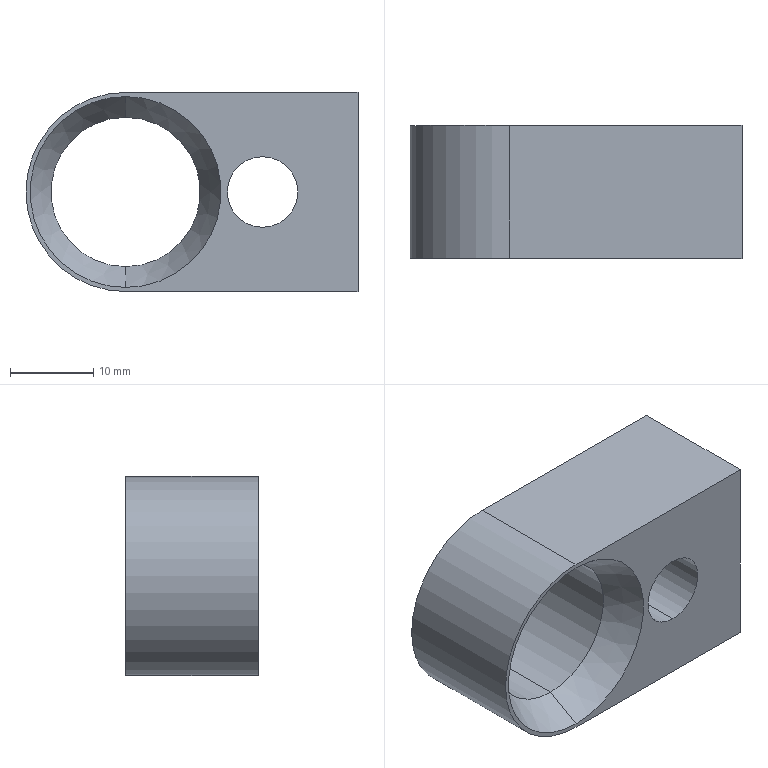Part | 1 solid | 12 faces | box 40 x 16 x 24 mm | volume 9057 mm3 | cylinder 5 | plane 5 | cone 2 | commonest cylinder face diameters 8.5 x2 18 x2 24 x1
STEP:
#1=CARTESIAN_POINT('',(-8.,4.33,9.));
#2=VERTEX_POINT('',#1);
#3=CARTESIAN_POINT('',(-8.,4.33,-9.));
#4=VERTEX_POINT('',#3);
#5=CARTESIAN_POINT('',(-8.,4.33,0.));
#6=DIRECTION('',(0.,1.,0.));
#7=DIRECTION('',(0.,0.,-1.));
#8=AXIS2_PLACEMENT_3D('',#5,#6,#7);
#9=CIRCLE('',#8,9.);
#10=EDGE_CURVE('',#2,#4,#9,.T.);
#11=ORIENTED_EDGE('',*,*,#10,.T.);
#12=CARTESIAN_POINT('',(-8.,0.,-11.5));
#13=VERTEX_POINT('',#12);
#14=CARTESIAN_POINT('',(-8.,0.,-11.5));
#15=DIRECTION('',(0.,-0.866,-0.5));
#16=VECTOR('',#15,1000.);
#17=LINE('',#14,#16);
#18=EDGE_CURVE('',#4,#13,#17,.T.);
#19=ORIENTED_EDGE('',*,*,#18,.T.);
#20=CARTESIAN_POINT('',(-8.,0.,11.5));
#21=VERTEX_POINT('',#20);
#22=CARTESIAN_POINT('',(-8.,0.,0.));
#23=DIRECTION('',(0.,1.,0.));
#24=DIRECTION('',(0.,0.,1.));
#25=AXIS2_PLACEMENT_3D('',#22,#23,#24);
#26=CIRCLE('',#25,11.5);
#27=EDGE_CURVE('',#21,#13,#26,.T.);
#28=ORIENTED_EDGE('',*,*,#27,.F.);
#29=CARTESIAN_POINT('',(-8.,0.,11.5));
#30=DIRECTION('',(0.,-0.866,0.5));
#31=VECTOR('',#30,1000.);
#32=LINE('',#29,#31);
#33=EDGE_CURVE('',#2,#21,#32,.T.);
#34=ORIENTED_EDGE('',*,*,#33,.F.);
#35=EDGE_LOOP('',(#11,#19,#28,#34));
#36=FACE_OUTER_BOUND('',#35,.T.);
#37=CARTESIAN_POINT('',(-8.,0.,0.));
#38=DIRECTION('',(0.,-1.,0.));
#39=DIRECTION('',(0.,0.,1.));
#40=AXIS2_PLACEMENT_3D('',#37,#38,#39);
#41=CONICAL_SURFACE('',#40,11.5,0.5236);
#42=ADVANCED_FACE('',(#36),#41,.F.);
#43=CARTESIAN_POINT('',(8.5,0.,-4.25));
#44=VERTEX_POINT('',#43);
#45=CARTESIAN_POINT('',(8.5,0.,4.25));
#46=VERTEX_POINT('',#45);
#47=CARTESIAN_POINT('',(8.5,0.,0.));
#48=DIRECTION('',(0.,1.,0.));
#49=DIRECTION('',(0.,0.,1.));
#50=AXIS2_PLACEMENT_3D('',#47,#48,#49);
#51=CIRCLE('',#50,4.25);
#52=EDGE_CURVE('',#44,#46,#51,.T.);
#53=ORIENTED_EDGE('',*,*,#52,.F.);
#54=CARTESIAN_POINT('',(8.5,16.,-4.25));
#55=VERTEX_POINT('',#54);
#56=CARTESIAN_POINT('',(8.5,0.,-4.25));
#57=DIRECTION('',(0.,1.,0.));
#58=VECTOR('',#57,1000.);
#59=LINE('',#56,#58);
#60=EDGE_CURVE('',#44,#55,#59,.T.);
#61=ORIENTED_EDGE('',*,*,#60,.T.);
#62=CARTESIAN_POINT('',(8.5,16.,4.25));
#63=VERTEX_POINT('',#62);
#64=CARTESIAN_POINT('',(8.5,16.,0.));
#65=DIRECTION('',(0.,1.,0.));
#66=DIRECTION('',(0.,0.,1.));
#67=AXIS2_PLACEMENT_3D('',#64,#65,#66);
#68=CIRCLE('',#67,4.25);
#69=EDGE_CURVE('',#55,#63,#68,.T.);
#70=ORIENTED_EDGE('',*,*,#69,.T.);
#71=CARTESIAN_POINT('',(8.5,0.,4.25));
#72=DIRECTION('',(0.,1.,0.));
#73=VECTOR('',#72,1000.);
#74=LINE('',#71,#73);
#75=EDGE_CURVE('',#46,#63,#74,.T.);
#76=ORIENTED_EDGE('',*,*,#75,.F.);
#77=EDGE_LOOP('',(#53,#61,#70,#76));
#78=FACE_OUTER_BOUND('',#77,.T.);
#79=CARTESIAN_POINT('',(8.5,0.,0.));
#80=DIRECTION('',(0.,1.,0.));
#81=DIRECTION('',(0.,0.,1.));
#82=AXIS2_PLACEMENT_3D('',#79,#80,#81);
#83=CYLINDRICAL_SURFACE('',#82,4.25);
#84=ADVANCED_FACE('',(#78),#83,.F.);
#85=CARTESIAN_POINT('',(-8.,4.33,0.));
#86=DIRECTION('',(0.,1.,0.));
#87=DIRECTION('',(0.,0.,-1.));
#88=AXIS2_PLACEMENT_3D('',#85,#86,#87);
#89=CIRCLE('',#88,9.);
#90=EDGE_CURVE('',#4,#2,#89,.T.);
#91=ORIENTED_EDGE('',*,*,#90,.F.);
#92=CARTESIAN_POINT('',(-8.,16.,-9.));
#93=VERTEX_POINT('',#92);
#94=CARTESIAN_POINT('',(-8.,0.,-9.));
#95=DIRECTION('',(0.,1.,0.));
#96=VECTOR('',#95,1000.);
#97=LINE('',#94,#96);
#98=EDGE_CURVE('',#4,#93,#97,.T.);
#99=ORIENTED_EDGE('',*,*,#98,.T.);
#100=CARTESIAN_POINT('',(-8.,16.,9.));
#101=VERTEX_POINT('',#100);
#102=CARTESIAN_POINT('',(-8.,16.,0.));
#103=DIRECTION('',(0.,1.,0.));
#104=DIRECTION('',(0.,0.,1.));
#105=AXIS2_PLACEMENT_3D('',#102,#103,#104);
#106=CIRCLE('',#105,9.);
#107=EDGE_CURVE('',#93,#101,#106,.T.);
#108=ORIENTED_EDGE('',*,*,#107,.T.);
#109=CARTESIAN_POINT('',(-8.,0.,9.));
#110=DIRECTION('',(0.,1.,0.));
#111=VECTOR('',#110,1000.);
#112=LINE('',#109,#111);
#113=EDGE_CURVE('',#2,#101,#112,.T.);
#114=ORIENTED_EDGE('',*,*,#113,.F.);
#115=EDGE_LOOP('',(#91,#99,#108,#114));
#116=FACE_OUTER_BOUND('',#115,.T.);
#117=CARTESIAN_POINT('',(-8.,0.,0.));
#118=DIRECTION('',(0.,1.,0.));
#119=DIRECTION('',(0.,0.,1.));
#120=AXIS2_PLACEMENT_3D('',#117,#118,#119);
#121=CYLINDRICAL_SURFACE('',#120,9.);
#122=ADVANCED_FACE('',(#116),#121,.F.);
#123=ORIENTED_EDGE('',*,*,#98,.F.);
#124=ORIENTED_EDGE('',*,*,#10,.F.);
#125=ORIENTED_EDGE('',*,*,#113,.T.);
#126=CARTESIAN_POINT('',(-8.,16.,0.));
#127=DIRECTION('',(0.,1.,0.));
#128=DIRECTION('',(0.,0.,1.));
#129=AXIS2_PLACEMENT_3D('',#126,#127,#128);
#130=CIRCLE('',#129,9.);
#131=EDGE_CURVE('',#101,#93,#130,.T.);
#132=ORIENTED_EDGE('',*,*,#131,.T.);
#133=EDGE_LOOP('',(#123,#124,#125,#132));
#134=FACE_OUTER_BOUND('',#133,.T.);
#135=CARTESIAN_POINT('',(-8.,0.,0.));
#136=DIRECTION('',(0.,1.,0.));
#137=DIRECTION('',(0.,0.,1.));
#138=AXIS2_PLACEMENT_3D('',#135,#136,#137);
#139=CYLINDRICAL_SURFACE('',#138,9.);
#140=ADVANCED_FACE('',(#134),#139,.F.);
#141=CARTESIAN_POINT('',(8.5,16.,0.));
#142=DIRECTION('',(0.,1.,0.));
#143=DIRECTION('',(0.,0.,1.));
#144=AXIS2_PLACEMENT_3D('',#141,#142,#143);
#145=CIRCLE('',#144,4.25);
#146=EDGE_CURVE('',#63,#55,#145,.T.);
#147=ORIENTED_EDGE('',*,*,#146,.F.);
#148=ORIENTED_EDGE('',*,*,#69,.F.);
#149=EDGE_LOOP('',(#147,#148));
#150=FACE_BOUND('',#149,.T.);
#151=ORIENTED_EDGE('',*,*,#131,.F.);
#152=ORIENTED_EDGE('',*,*,#107,.F.);
#153=EDGE_LOOP('',(#151,#152));
#154=FACE_BOUND('',#153,.T.);
#155=CARTESIAN_POINT('',(-8.,16.,-12.));
#156=VERTEX_POINT('',#155);
#157=CARTESIAN_POINT('',(-8.,16.,12.));
#158=VERTEX_POINT('',#157);
#159=CARTESIAN_POINT('',(-8.,16.,0.));
#160=DIRECTION('',(0.,1.,0.));
#161=DIRECTION('',(0.,0.,1.));
#162=AXIS2_PLACEMENT_3D('',#159,#160,#161);
#163=CIRCLE('',#162,12.);
#164=EDGE_CURVE('',#156,#158,#163,.T.);
#165=ORIENTED_EDGE('',*,*,#164,.T.);
#166=CARTESIAN_POINT('',(20.,16.,12.));
#167=VERTEX_POINT('',#166);
#168=CARTESIAN_POINT('',(-20.,16.,12.));
#169=DIRECTION('',(1.,0.,0.));
#170=VECTOR('',#169,1000.);
#171=LINE('',#168,#170);
#172=EDGE_CURVE('',#158,#167,#171,.T.);
#173=ORIENTED_EDGE('',*,*,#172,.T.);
#174=CARTESIAN_POINT('',(20.,16.,-12.));
#175=VERTEX_POINT('',#174);
#176=CARTESIAN_POINT('',(20.,16.,12.));
#177=DIRECTION('',(0.,0.,-1.));
#178=VECTOR('',#177,1000.);
#179=LINE('',#176,#178);
#180=EDGE_CURVE('',#167,#175,#179,.T.);
#181=ORIENTED_EDGE('',*,*,#180,.T.);
#182=CARTESIAN_POINT('',(-20.,16.,-12.));
#183=DIRECTION('',(-1.,0.,0.));
#184=VECTOR('',#183,1000.);
#185=LINE('',#182,#184);
#186=EDGE_CURVE('',#175,#156,#185,.T.);
#187=ORIENTED_EDGE('',*,*,#186,.T.);
#188=EDGE_LOOP('',(#165,#173,#181,#187));
#189=FACE_OUTER_BOUND('',#188,.T.);
#190=CARTESIAN_POINT('',(0.,16.,0.));
#191=DIRECTION('',(0.,-1.,0.));
#192=DIRECTION('',(0.,0.,-1.));
#193=AXIS2_PLACEMENT_3D('',#190,#191,#192);
#194=PLANE('',#193);
#195=ADVANCED_FACE('',(#150,#154,#189),#194,.F.);
#196=ORIENTED_EDGE('',*,*,#27,.T.);
#197=CARTESIAN_POINT('',(-8.,0.,0.));
#198=DIRECTION('',(0.,1.,0.));
#199=DIRECTION('',(0.,0.,1.));
#200=AXIS2_PLACEMENT_3D('',#197,#198,#199);
#201=CIRCLE('',#200,11.5);
#202=EDGE_CURVE('',#13,#21,#201,.T.);
#203=ORIENTED_EDGE('',*,*,#202,.T.);
#204=EDGE_LOOP('',(#196,#203));
#205=FACE_BOUND('',#204,.T.);
#206=CARTESIAN_POINT('',(8.5,0.,0.));
#207=DIRECTION('',(0.,1.,0.));
#208=DIRECTION('',(0.,0.,1.));
#209=AXIS2_PLACEMENT_3D('',#206,#207,#208);
#210=CIRCLE('',#209,4.25);
#211=EDGE_CURVE('',#46,#44,#210,.T.);
#212=ORIENTED_EDGE('',*,*,#211,.T.);
#213=ORIENTED_EDGE('',*,*,#52,.T.);
#214=EDGE_LOOP('',(#212,#213));
#215=FACE_BOUND('',#214,.T.);
#216=CARTESIAN_POINT('',(-8.,0.,12.));
#217=VERTEX_POINT('',#216);
#218=CARTESIAN_POINT('',(20.,0.,12.));
#219=VERTEX_POINT('',#218);
#220=CARTESIAN_POINT('',(-20.,0.,12.));
#221=DIRECTION('',(1.,0.,0.));
#222=VECTOR('',#221,1000.);
#223=LINE('',#220,#222);
#224=EDGE_CURVE('',#217,#219,#223,.T.);
#225=ORIENTED_EDGE('',*,*,#224,.F.);
#226=CARTESIAN_POINT('',(-8.,0.,-12.));
#227=VERTEX_POINT('',#226);
#228=CARTESIAN_POINT('',(-8.,0.,0.));
#229=DIRECTION('',(0.,1.,0.));
#230=DIRECTION('',(0.,0.,1.));
#231=AXIS2_PLACEMENT_3D('',#228,#229,#230);
#232=CIRCLE('',#231,12.);
#233=EDGE_CURVE('',#227,#217,#232,.T.);
#234=ORIENTED_EDGE('',*,*,#233,.F.);
#235=CARTESIAN_POINT('',(20.,0.,-12.));
#236=VERTEX_POINT('',#235);
#237=CARTESIAN_POINT('',(-20.,0.,-12.));
#238=DIRECTION('',(-1.,0.,0.));
#239=VECTOR('',#238,1000.);
#240=LINE('',#237,#239);
#241=EDGE_CURVE('',#236,#227,#240,.T.);
#242=ORIENTED_EDGE('',*,*,#241,.F.);
#243=CARTESIAN_POINT('',(20.,0.,12.));
#244=DIRECTION('',(0.,0.,-1.));
#245=VECTOR('',#244,1000.);
#246=LINE('',#243,#245);
#247=EDGE_CURVE('',#219,#236,#246,.T.);
#248=ORIENTED_EDGE('',*,*,#247,.F.);
#249=EDGE_LOOP('',(#225,#234,#242,#248));
#250=FACE_OUTER_BOUND('',#249,.T.);
#251=CARTESIAN_POINT('',(0.,0.,0.));
#252=DIRECTION('',(0.,-1.,0.));
#253=DIRECTION('',(0.,0.,-1.));
#254=AXIS2_PLACEMENT_3D('',#251,#252,#253);
#255=PLANE('',#254);
#256=ADVANCED_FACE('',(#205,#215,#250),#255,.T.);
#257=CARTESIAN_POINT('',(-8.,0.,12.));
#258=DIRECTION('',(0.,1.,0.));
#259=VECTOR('',#258,1000.);
#260=LINE('',#257,#259);
#261=EDGE_CURVE('',#217,#158,#260,.T.);
#262=ORIENTED_EDGE('',*,*,#261,.F.);
#263=ORIENTED_EDGE('',*,*,#224,.T.);
#264=CARTESIAN_POINT('',(20.,16.,12.));
#265=DIRECTION('',(0.,-1.,0.));
#266=VECTOR('',#265,1000.);
#267=LINE('',#264,#266);
#268=EDGE_CURVE('',#167,#219,#267,.T.);
#269=ORIENTED_EDGE('',*,*,#268,.F.);
#270=ORIENTED_EDGE('',*,*,#172,.F.);
#271=EDGE_LOOP('',(#262,#263,#269,#270));
#272=FACE_OUTER_BOUND('',#271,.T.);
#273=CARTESIAN_POINT('',(-20.,16.,12.));
#274=DIRECTION('',(0.,0.,-1.));
#275=DIRECTION('',(-1.,0.,0.));
#276=AXIS2_PLACEMENT_3D('',#273,#274,#275);
#277=PLANE('',#276);
#278=ADVANCED_FACE('',(#272),#277,.F.);
#279=ORIENTED_EDGE('',*,*,#247,.T.);
#280=CARTESIAN_POINT('',(20.,16.,-12.));
#281=DIRECTION('',(0.,-1.,0.));
#282=VECTOR('',#281,1000.);
#283=LINE('',#280,#282);
#284=EDGE_CURVE('',#175,#236,#283,.T.);
#285=ORIENTED_EDGE('',*,*,#284,.F.);
#286=ORIENTED_EDGE('',*,*,#180,.F.);
#287=ORIENTED_EDGE('',*,*,#268,.T.);
#288=EDGE_LOOP('',(#279,#285,#286,#287));
#289=FACE_OUTER_BOUND('',#288,.T.);
#290=CARTESIAN_POINT('',(20.,16.,12.));
#291=DIRECTION('',(-1.,0.,0.));
#292=DIRECTION('',(0.,0.,1.));
#293=AXIS2_PLACEMENT_3D('',#290,#291,#292);
#294=PLANE('',#293);
#295=ADVANCED_FACE('',(#289),#294,.F.);
#296=ORIENTED_EDGE('',*,*,#241,.T.);
#297=CARTESIAN_POINT('',(-8.,0.,-12.));
#298=DIRECTION('',(0.,1.,0.));
#299=VECTOR('',#298,1000.);
#300=LINE('',#297,#299);
#301=EDGE_CURVE('',#227,#156,#300,.T.);
#302=ORIENTED_EDGE('',*,*,#301,.T.);
#303=ORIENTED_EDGE('',*,*,#186,.F.);
#304=ORIENTED_EDGE('',*,*,#284,.T.);
#305=EDGE_LOOP('',(#296,#302,#303,#304));
#306=FACE_OUTER_BOUND('',#305,.T.);
#307=CARTESIAN_POINT('',(-20.,16.,-12.));
#308=DIRECTION('',(0.,0.,1.));
#309=DIRECTION('',(1.,0.,0.));
#310=AXIS2_PLACEMENT_3D('',#307,#308,#309);
#311=PLANE('',#310);
#312=ADVANCED_FACE('',(#306),#311,.F.);
#313=ORIENTED_EDGE('',*,*,#164,.F.);
#314=ORIENTED_EDGE('',*,*,#301,.F.);
#315=ORIENTED_EDGE('',*,*,#233,.T.);
#316=ORIENTED_EDGE('',*,*,#261,.T.);
#317=EDGE_LOOP('',(#313,#314,#315,#316));
#318=FACE_OUTER_BOUND('',#317,.T.);
#319=CARTESIAN_POINT('',(-8.,0.,0.));
#320=DIRECTION('',(0.,1.,0.));
#321=DIRECTION('',(0.,0.,1.));
#322=AXIS2_PLACEMENT_3D('',#319,#320,#321);
#323=CYLINDRICAL_SURFACE('',#322,12.);
#324=ADVANCED_FACE('',(#318),#323,.T.);
#325=ORIENTED_EDGE('',*,*,#60,.F.);
#326=ORIENTED_EDGE('',*,*,#211,.F.);
#327=ORIENTED_EDGE('',*,*,#75,.T.);
#328=ORIENTED_EDGE('',*,*,#146,.T.);
#329=EDGE_LOOP('',(#325,#326,#327,#328));
#330=FACE_OUTER_BOUND('',#329,.T.);
#331=CARTESIAN_POINT('',(8.5,0.,0.));
#332=DIRECTION('',(0.,1.,0.));
#333=DIRECTION('',(0.,0.,1.));
#334=AXIS2_PLACEMENT_3D('',#331,#332,#333);
#335=CYLINDRICAL_SURFACE('',#334,4.25);
#336=ADVANCED_FACE('',(#330),#335,.F.);
#337=ORIENTED_EDGE('',*,*,#18,.F.);
#338=ORIENTED_EDGE('',*,*,#90,.T.);
#339=ORIENTED_EDGE('',*,*,#33,.T.);
#340=ORIENTED_EDGE('',*,*,#202,.F.);
#341=EDGE_LOOP('',(#337,#338,#339,#340));
#342=FACE_OUTER_BOUND('',#341,.T.);
#343=CARTESIAN_POINT('',(-8.,0.,0.));
#344=DIRECTION('',(0.,-1.,0.));
#345=DIRECTION('',(0.,0.,1.));
#346=AXIS2_PLACEMENT_3D('',#343,#344,#345);
#347=CONICAL_SURFACE('',#346,11.5,0.5236);
#348=ADVANCED_FACE('',(#342),#347,.F.);
#349=CLOSED_SHELL('',(#42,#84,#122,#140,#195,#256,#278,#295,#312,#324,#336,#348));
#350=MANIFOLD_SOLID_BREP('',#349);
#351=CARTESIAN_POINT('',(0.,0.,0.));
#352=DIRECTION('',(0.,0.,1.));
#353=DIRECTION('',(1.,0.,0.));
#354=AXIS2_PLACEMENT_3D('',#351,#352,#353);
#355=(LENGTH_UNIT()NAMED_UNIT(*)SI_UNIT(.MILLI.,.METRE.));
#356=UNCERTAINTY_MEASURE_WITH_UNIT(LENGTH_MEASURE(0.00001),#355,'','');
#357=(NAMED_UNIT(*)PLANE_ANGLE_UNIT()SI_UNIT($,.RADIAN.));
#358=(NAMED_UNIT(*)SI_UNIT($,.STERADIAN.)SOLID_ANGLE_UNIT());
#359=(GEOMETRIC_REPRESENTATION_CONTEXT(3)GLOBAL_UNCERTAINTY_ASSIGNED_CONTEXT((#356))GLOBAL_UNIT_ASSIGNED_CONTEXT((#355,#357,#358))REPRESENTATION_CONTEXT('',''));
#360=ADVANCED_BREP_SHAPE_REPRESENTATION('',(#350,#354),#359);